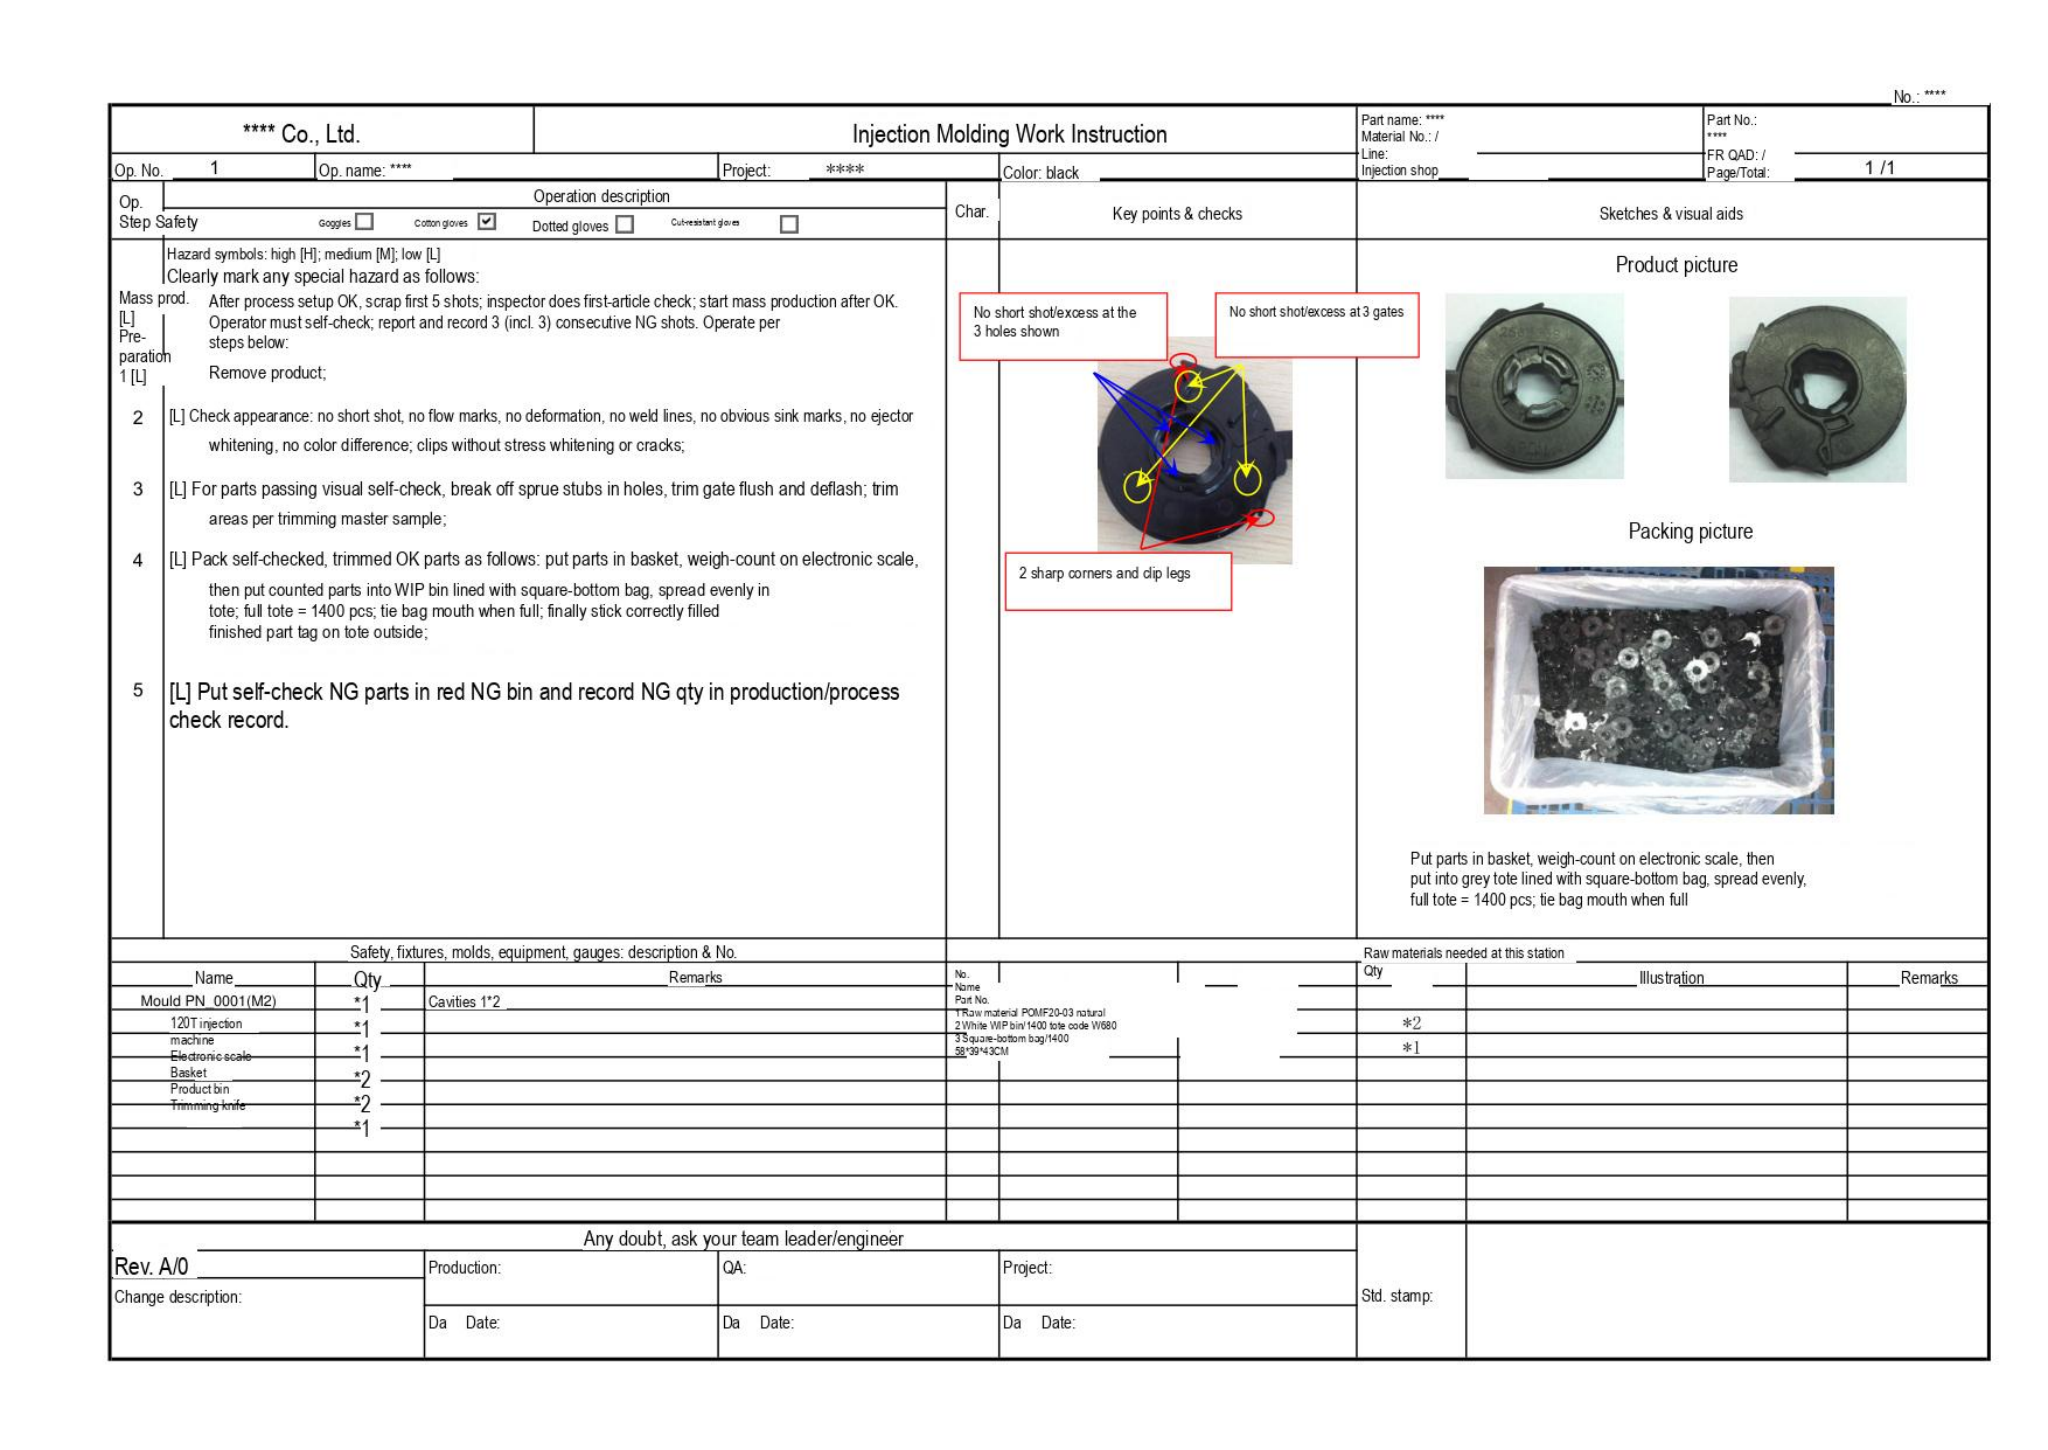No.: ****

| **** Co., Ltd. | Injection Molding Work Instruction | Part name: ****<br>Material No.: /<br>Line:<br>Injection shop | Part No.:<br>****<br>FR QAD: /<br>Page/Total: 1 /1 |
|---|---|---|---|

| Op. No. 1 | Op. name: **** | Project: **** | Color: black |
|---|---|---|---|

| Op. Step | Safety | Operation description | Char. | Key points & checks | Sketches & visual aids |
|---|---|---|---|---|---|
| | Goggles ☐ Cotton gloves ☑ Dotted gloves ☐ Cut-resistant gloves ☐ | Hazard symbols: high [H]; medium [M]; low [L]<br>Clearly mark any special hazard as follows: | | | |
| Mass prod. [L] Pre-paration 1 [L] | | After process setup OK, scrap first 5 shots; inspector does first-article check; start mass production after OK. Operator must self-check; report and record 3 (incl. 3) consecutive NG shots. Operate per steps below:<br>Remove product; | | No short shot/excess at the 3 holes shown<br>No short shot/excess at 3 gates<br>2 sharp corners and clip legs | Product picture |
| 2 | | [L] Check appearance: no short shot, no flow marks, no deformation, no weld lines, no obvious sink marks, no ejector whitening, no color difference; clips without stress whitening or cracks; | | | |
| 3 | | [L] For parts passing visual self-check, break off sprue stubs in holes, trim gate flush and deflash; trim areas per trimming master sample; | | | Packing picture |
| 4 | | [L] Pack self-checked, trimmed OK parts as follows: put parts in basket, weigh-count on electronic scale, then put counted parts into WIP bin lined with square-bottom bag, spread evenly in tote; full tote = 1400 pcs; tie bag mouth when full; finally stick correctly filled finished part tag on tote outside; | | | |
| 5 | | [L] Put self-check NG parts in red NG bin and record NG qty in production/process check record. | | | Put parts in basket, weigh-count on electronic scale, then put into grey tote lined with square-bottom bag, spread evenly, full tote = 1400 pcs; tie bag mouth when full |

Safety, fixtures, molds, equipment, gauges: description & No.

| Name | Qty | Remarks |
|---|---|---|
| Mould PN_0001(M2) | *1 | Cavities 1*2 |
| 120T injection machine | *1 | |
| Electronic scale | *1 | |
| Basket | *2 | |
| Product bin | *2 | |
| Trimming knife | *1 | |

Raw materials needed at this station

| No. Name Part No. | Qty | Illustration | Remarks |
|---|---|---|---|
| 1 Raw material POMF20-03 natural | | | |
| 2 White WIP bin/1400 tote code W680 | *2 | | |
| 3 Square-bottom bag/1400 58*39*43CM | *1 | | |

Any doubt, ask your team leader/engineer

| Rev. A/0<br>Change description: | Production:<br>Da Date: | QA:<br>Da Date: | Project:<br>Da Date: | Std. stamp: |
|---|---|---|---|---|